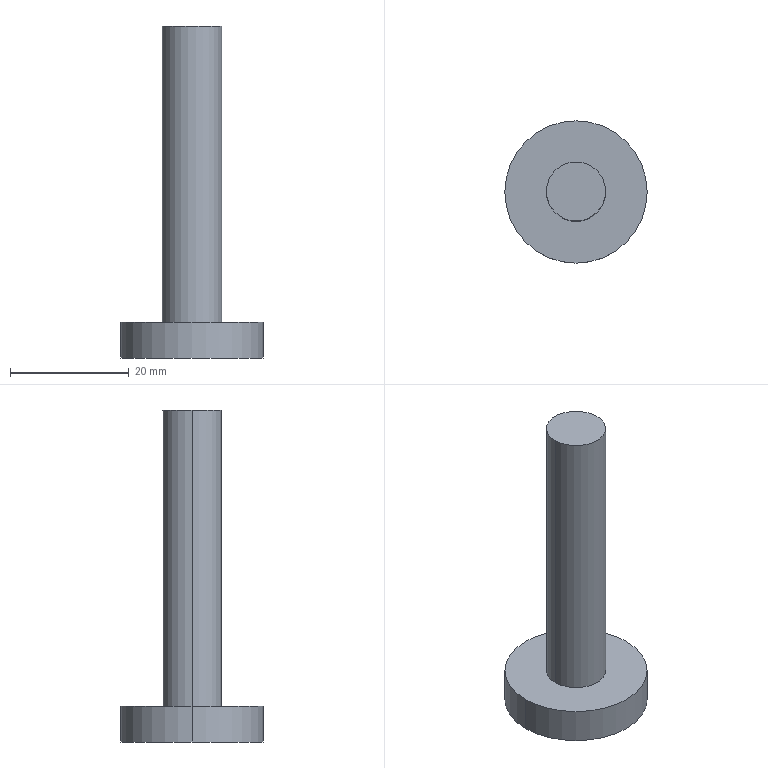Part | SolidWorks | features Extrusion 1, ICE 1 | 1 solid | 7 faces | box 24 x 24 x 56 mm | volume 6641 mm3 | cylinder 4 | plane 3 | commonest cylinder face diameters 10 x2 24 x2
STEP:
#1=CARTESIAN_POINT('',(12.,0.,-6.));
#2=VERTEX_POINT('',#1);
#3=CARTESIAN_POINT('',(-12.,0.,-6.));
#4=VERTEX_POINT('',#3);
#5=CARTESIAN_POINT('',(0.,0.,-6.));
#6=DIRECTION('',(0.,0.,1.));
#7=DIRECTION('',(1.,0.,0.));
#8=AXIS2_PLACEMENT_3D('',#5,#6,#7);
#9=CIRCLE('',#8,12.);
#10=EDGE_CURVE('',#2,#4,#9,.T.);
#11=ORIENTED_EDGE('',*,*,#10,.T.);
#12=CARTESIAN_POINT('',(-12.,0.,0.));
#13=VERTEX_POINT('',#12);
#14=CARTESIAN_POINT('',(-12.,0.,-6.));
#15=DIRECTION('',(0.,0.,1.));
#16=VECTOR('',#15,1000.);
#17=LINE('',#14,#16);
#18=EDGE_CURVE('',#4,#13,#17,.T.);
#19=ORIENTED_EDGE('',*,*,#18,.T.);
#20=CARTESIAN_POINT('',(12.,0.,0.));
#21=VERTEX_POINT('',#20);
#22=CARTESIAN_POINT('',(0.,0.,0.));
#23=DIRECTION('',(0.,0.,1.));
#24=DIRECTION('',(1.,0.,0.));
#25=AXIS2_PLACEMENT_3D('',#22,#23,#24);
#26=CIRCLE('',#25,12.);
#27=EDGE_CURVE('',#21,#13,#26,.T.);
#28=ORIENTED_EDGE('',*,*,#27,.F.);
#29=CARTESIAN_POINT('',(12.,0.,-6.));
#30=DIRECTION('',(0.,0.,1.));
#31=VECTOR('',#30,1000.);
#32=LINE('',#29,#31);
#33=EDGE_CURVE('',#2,#21,#32,.T.);
#34=ORIENTED_EDGE('',*,*,#33,.F.);
#35=EDGE_LOOP('',(#11,#19,#28,#34));
#36=FACE_OUTER_BOUND('',#35,.T.);
#37=CARTESIAN_POINT('',(0.,0.,-6.));
#38=DIRECTION('',(0.,0.,1.));
#39=DIRECTION('',(1.,0.,0.));
#40=AXIS2_PLACEMENT_3D('',#37,#38,#39);
#41=CYLINDRICAL_SURFACE('',#40,12.);
#42=ADVANCED_FACE('',(#36),#41,.T.);
#43=CARTESIAN_POINT('',(5.,0.,50.));
#44=VERTEX_POINT('',#43);
#45=CARTESIAN_POINT('',(-5.,0.,50.));
#46=VERTEX_POINT('',#45);
#47=CARTESIAN_POINT('',(0.,0.,50.));
#48=DIRECTION('',(0.,0.,1.));
#49=DIRECTION('',(1.,0.,0.));
#50=AXIS2_PLACEMENT_3D('',#47,#48,#49);
#51=CIRCLE('',#50,5.);
#52=EDGE_CURVE('',#44,#46,#51,.T.);
#53=ORIENTED_EDGE('',*,*,#52,.F.);
#54=CARTESIAN_POINT('',(5.,0.,0.));
#55=VERTEX_POINT('',#54);
#56=CARTESIAN_POINT('',(5.,0.,50.));
#57=DIRECTION('',(0.,0.,-1.));
#58=VECTOR('',#57,1000.);
#59=LINE('',#56,#58);
#60=EDGE_CURVE('',#44,#55,#59,.T.);
#61=ORIENTED_EDGE('',*,*,#60,.T.);
#62=CARTESIAN_POINT('',(-5.,0.,0.));
#63=VERTEX_POINT('',#62);
#64=CARTESIAN_POINT('',(0.,0.,0.));
#65=DIRECTION('',(0.,0.,1.));
#66=DIRECTION('',(1.,0.,0.));
#67=AXIS2_PLACEMENT_3D('',#64,#65,#66);
#68=CIRCLE('',#67,5.);
#69=EDGE_CURVE('',#55,#63,#68,.T.);
#70=ORIENTED_EDGE('',*,*,#69,.T.);
#71=CARTESIAN_POINT('',(-5.,0.,50.));
#72=DIRECTION('',(0.,0.,-1.));
#73=VECTOR('',#72,1000.);
#74=LINE('',#71,#73);
#75=EDGE_CURVE('',#46,#63,#74,.T.);
#76=ORIENTED_EDGE('',*,*,#75,.F.);
#77=EDGE_LOOP('',(#53,#61,#70,#76));
#78=FACE_OUTER_BOUND('',#77,.T.);
#79=CARTESIAN_POINT('',(0.,0.,50.));
#80=DIRECTION('',(0.,0.,-1.));
#81=DIRECTION('',(-1.,0.,0.));
#82=AXIS2_PLACEMENT_3D('',#79,#80,#81);
#83=CYLINDRICAL_SURFACE('',#82,5.);
#84=ADVANCED_FACE('',(#78),#83,.T.);
#85=ORIENTED_EDGE('',*,*,#60,.F.);
#86=CARTESIAN_POINT('',(0.,0.,50.));
#87=DIRECTION('',(0.,0.,1.));
#88=DIRECTION('',(1.,0.,0.));
#89=AXIS2_PLACEMENT_3D('',#86,#87,#88);
#90=CIRCLE('',#89,5.);
#91=EDGE_CURVE('',#46,#44,#90,.T.);
#92=ORIENTED_EDGE('',*,*,#91,.F.);
#93=ORIENTED_EDGE('',*,*,#75,.T.);
#94=CARTESIAN_POINT('',(0.,0.,0.));
#95=DIRECTION('',(0.,0.,1.));
#96=DIRECTION('',(1.,0.,0.));
#97=AXIS2_PLACEMENT_3D('',#94,#95,#96);
#98=CIRCLE('',#97,5.);
#99=EDGE_CURVE('',#63,#55,#98,.T.);
#100=ORIENTED_EDGE('',*,*,#99,.T.);
#101=EDGE_LOOP('',(#85,#92,#93,#100));
#102=FACE_OUTER_BOUND('',#101,.T.);
#103=CARTESIAN_POINT('',(0.,0.,50.));
#104=DIRECTION('',(0.,0.,-1.));
#105=DIRECTION('',(-1.,0.,0.));
#106=AXIS2_PLACEMENT_3D('',#103,#104,#105);
#107=CYLINDRICAL_SURFACE('',#106,5.);
#108=ADVANCED_FACE('',(#102),#107,.T.);
#109=ORIENTED_EDGE('',*,*,#91,.T.);
#110=ORIENTED_EDGE('',*,*,#52,.T.);
#111=EDGE_LOOP('',(#109,#110));
#112=FACE_OUTER_BOUND('',#111,.T.);
#113=CARTESIAN_POINT('',(0.,0.,50.));
#114=DIRECTION('',(0.,0.,1.));
#115=DIRECTION('',(1.,0.,0.));
#116=AXIS2_PLACEMENT_3D('',#113,#114,#115);
#117=PLANE('',#116);
#118=ADVANCED_FACE('',(#112),#117,.T.);
#119=ORIENTED_EDGE('',*,*,#18,.F.);
#120=CARTESIAN_POINT('',(0.,0.,-6.));
#121=DIRECTION('',(0.,0.,1.));
#122=DIRECTION('',(1.,0.,0.));
#123=AXIS2_PLACEMENT_3D('',#120,#121,#122);
#124=CIRCLE('',#123,12.);
#125=EDGE_CURVE('',#4,#2,#124,.T.);
#126=ORIENTED_EDGE('',*,*,#125,.T.);
#127=ORIENTED_EDGE('',*,*,#33,.T.);
#128=CARTESIAN_POINT('',(0.,0.,0.));
#129=DIRECTION('',(0.,0.,1.));
#130=DIRECTION('',(1.,0.,0.));
#131=AXIS2_PLACEMENT_3D('',#128,#129,#130);
#132=CIRCLE('',#131,12.);
#133=EDGE_CURVE('',#13,#21,#132,.T.);
#134=ORIENTED_EDGE('',*,*,#133,.F.);
#135=EDGE_LOOP('',(#119,#126,#127,#134));
#136=FACE_OUTER_BOUND('',#135,.T.);
#137=CARTESIAN_POINT('',(0.,0.,-6.));
#138=DIRECTION('',(0.,0.,1.));
#139=DIRECTION('',(1.,0.,0.));
#140=AXIS2_PLACEMENT_3D('',#137,#138,#139);
#141=CYLINDRICAL_SURFACE('',#140,12.);
#142=ADVANCED_FACE('',(#136),#141,.T.);
#143=ORIENTED_EDGE('',*,*,#10,.F.);
#144=ORIENTED_EDGE('',*,*,#125,.F.);
#145=EDGE_LOOP('',(#143,#144));
#146=FACE_OUTER_BOUND('',#145,.T.);
#147=CARTESIAN_POINT('',(0.,0.,-6.));
#148=DIRECTION('',(0.,0.,1.));
#149=DIRECTION('',(1.,0.,0.));
#150=AXIS2_PLACEMENT_3D('',#147,#148,#149);
#151=PLANE('',#150);
#152=ADVANCED_FACE('',(#146),#151,.F.);
#153=ORIENTED_EDGE('',*,*,#99,.F.);
#154=ORIENTED_EDGE('',*,*,#69,.F.);
#155=EDGE_LOOP('',(#153,#154));
#156=FACE_BOUND('',#155,.T.);
#157=ORIENTED_EDGE('',*,*,#27,.T.);
#158=ORIENTED_EDGE('',*,*,#133,.T.);
#159=EDGE_LOOP('',(#157,#158));
#160=FACE_OUTER_BOUND('',#159,.T.);
#161=CARTESIAN_POINT('',(0.,0.,0.));
#162=DIRECTION('',(0.,0.,1.));
#163=DIRECTION('',(1.,0.,0.));
#164=AXIS2_PLACEMENT_3D('',#161,#162,#163);
#165=PLANE('',#164);
#166=ADVANCED_FACE('',(#156,#160),#165,.T.);
#167=CLOSED_SHELL('',(#42,#84,#108,#118,#142,#152,#166));
#168=MANIFOLD_SOLID_BREP('',#167);
#169=CARTESIAN_POINT('',(0.,0.,0.));
#170=DIRECTION('',(0.,0.,1.));
#171=DIRECTION('',(1.,0.,0.));
#172=AXIS2_PLACEMENT_3D('',#169,#170,#171);
#173=(LENGTH_UNIT()NAMED_UNIT(*)SI_UNIT(.MILLI.,.METRE.));
#174=UNCERTAINTY_MEASURE_WITH_UNIT(LENGTH_MEASURE(0.00001),#173,'','');
#175=(NAMED_UNIT(*)PLANE_ANGLE_UNIT()SI_UNIT($,.RADIAN.));
#176=(NAMED_UNIT(*)SI_UNIT($,.STERADIAN.)SOLID_ANGLE_UNIT());
#177=(GEOMETRIC_REPRESENTATION_CONTEXT(3)GLOBAL_UNCERTAINTY_ASSIGNED_CONTEXT((#174))GLOBAL_UNIT_ASSIGNED_CONTEXT((#173,#175,#176))REPRESENTATION_CONTEXT('',''));
#178=ADVANCED_BREP_SHAPE_REPRESENTATION('',(#168,#172),#177);